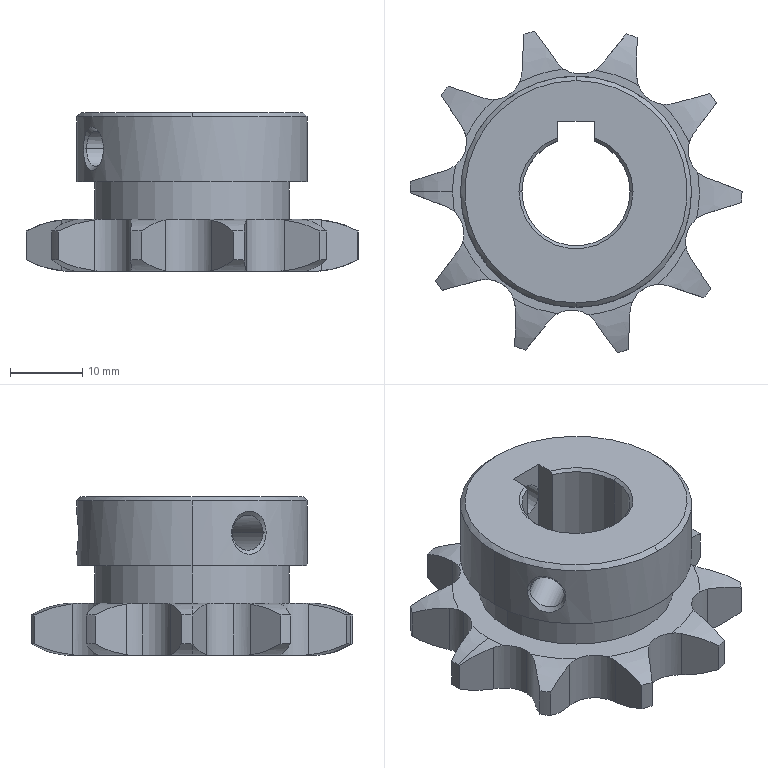Part | STEP file | 1.6米VLF02-40-10-D15 | 1 solid | 96 faces | box 46 x 44.551 x 22 mm | volume 14102 mm3 | cylinder 35 | plane 27 | spline 22 | cone 12 | commonest cylinder face diameters 8.04 x13 46 x11 4.917 x4 15 x3 27 x2 32 x2